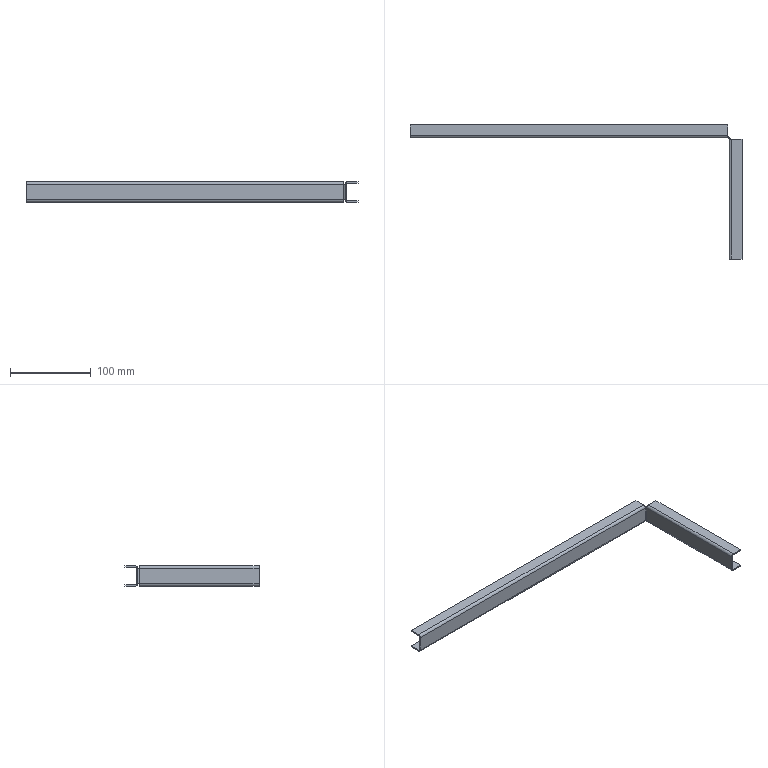Part | NX | features solid 2 | 1 solid | 34 faces | box 411 x 166 x 25 mm | volume 42432 mm3 | plane 24 | cylinder 10 | commonest cylinder face diameters 3 x5 6 x5
STEP:
#1=CARTESIAN_POINT('',(1091.,510.5,389.));
#2=VERTEX_POINT('',#1);
#3=CARTESIAN_POINT('',(1091.,509.,390.5));
#4=VERTEX_POINT('',#3);
#5=CARTESIAN_POINT('',(1091.,510.5,390.5));
#6=DIRECTION('',(-1.,0.,0.));
#7=DIRECTION('',(0.,0.,1.));
#8=AXIS2_PLACEMENT_3D('',#5,#6,#7);
#9=CIRCLE('',#8,1.5);
#10=EDGE_CURVE('',#2,#4,#9,.T.);
#11=ORIENTED_EDGE('',*,*,#10,.F.);
#12=CARTESIAN_POINT('',(697.5,510.5,389.));
#13=VERTEX_POINT('',#12);
#14=CARTESIAN_POINT('',(1091.,510.5,389.));
#15=DIRECTION('',(-1.,0.,0.));
#16=VECTOR('',#15,1000.);
#17=LINE('',#14,#16);
#18=EDGE_CURVE('',#2,#13,#17,.T.);
#19=ORIENTED_EDGE('',*,*,#18,.T.);
#20=CARTESIAN_POINT('',(697.5,509.,390.5));
#21=VERTEX_POINT('',#20);
#22=CARTESIAN_POINT('',(697.5,510.5,390.5));
#23=DIRECTION('',(1.,0.,0.));
#24=DIRECTION('',(0.,0.,1.));
#25=AXIS2_PLACEMENT_3D('',#22,#23,#24);
#26=CIRCLE('',#25,1.5);
#27=EDGE_CURVE('',#21,#13,#26,.T.);
#28=ORIENTED_EDGE('',*,*,#27,.F.);
#29=CARTESIAN_POINT('',(697.5,509.,390.5));
#30=DIRECTION('',(1.,0.,0.));
#31=VECTOR('',#30,1000.);
#32=LINE('',#29,#31);
#33=EDGE_CURVE('',#21,#4,#32,.T.);
#34=ORIENTED_EDGE('',*,*,#33,.T.);
#35=EDGE_LOOP('',(#11,#19,#28,#34));
#36=FACE_BOUND('',#35,.T.);
#37=CARTESIAN_POINT('',(697.5,510.5,390.5));
#38=DIRECTION('',(-1.,0.,0.));
#39=DIRECTION('',(0.,1.,0.));
#40=AXIS2_PLACEMENT_3D('',#37,#38,#39);
#41=CYLINDRICAL_SURFACE('',#40,1.5);
#42=ADVANCED_FACE('',(#36),#41,.F.);
#43=CARTESIAN_POINT('',(1091.,510.5,387.5));
#44=VERTEX_POINT('',#43);
#45=CARTESIAN_POINT('',(1091.,507.5,390.5));
#46=VERTEX_POINT('',#45);
#47=CARTESIAN_POINT('',(1091.,510.5,390.5));
#48=DIRECTION('',(-1.,0.,0.));
#49=DIRECTION('',(0.,1.,0.));
#50=AXIS2_PLACEMENT_3D('',#47,#48,#49);
#51=CIRCLE('',#50,3.);
#52=EDGE_CURVE('',#44,#46,#51,.T.);
#53=ORIENTED_EDGE('',*,*,#52,.T.);
#54=CARTESIAN_POINT('',(697.5,507.5,390.5));
#55=VERTEX_POINT('',#54);
#56=CARTESIAN_POINT('',(1091.,507.5,390.5));
#57=DIRECTION('',(1.,0.,0.));
#58=VECTOR('',#57,1000.);
#59=LINE('',#56,#58);
#60=EDGE_CURVE('',#55,#46,#59,.T.);
#61=ORIENTED_EDGE('',*,*,#60,.F.);
#62=CARTESIAN_POINT('',(697.5,510.5,387.5));
#63=VERTEX_POINT('',#62);
#64=CARTESIAN_POINT('',(697.5,510.5,390.5));
#65=DIRECTION('',(1.,0.,0.));
#66=DIRECTION('',(0.,1.,0.));
#67=AXIS2_PLACEMENT_3D('',#64,#65,#66);
#68=CIRCLE('',#67,3.);
#69=EDGE_CURVE('',#55,#63,#68,.T.);
#70=ORIENTED_EDGE('',*,*,#69,.T.);
#71=CARTESIAN_POINT('',(1091.,510.5,387.5));
#72=DIRECTION('',(-1.,0.,0.));
#73=VECTOR('',#72,1000.);
#74=LINE('',#71,#73);
#75=EDGE_CURVE('',#44,#63,#74,.T.);
#76=ORIENTED_EDGE('',*,*,#75,.F.);
#77=EDGE_LOOP('',(#53,#61,#70,#76));
#78=FACE_BOUND('',#77,.T.);
#79=CARTESIAN_POINT('',(697.5,510.5,390.5));
#80=DIRECTION('',(-1.,0.,0.));
#81=DIRECTION('',(0.,1.,0.));
#82=AXIS2_PLACEMENT_3D('',#79,#80,#81);
#83=CYLINDRICAL_SURFACE('',#82,3.);
#84=ADVANCED_FACE('',(#78),#83,.T.);
#85=CARTESIAN_POINT('',(697.5,523.5,389.));
#86=VERTEX_POINT('',#85);
#87=CARTESIAN_POINT('',(697.5,523.5,389.));
#88=DIRECTION('',(0.,-1.,0.));
#89=VECTOR('',#88,1000.);
#90=LINE('',#87,#89);
#91=EDGE_CURVE('',#86,#13,#90,.T.);
#92=ORIENTED_EDGE('',*,*,#91,.T.);
#93=ORIENTED_EDGE('',*,*,#18,.F.);
#94=CARTESIAN_POINT('',(1091.,523.5,389.));
#95=VERTEX_POINT('',#94);
#96=CARTESIAN_POINT('',(1091.,523.5,389.));
#97=DIRECTION('',(0.,-1.,0.));
#98=VECTOR('',#97,1000.);
#99=LINE('',#96,#98);
#100=EDGE_CURVE('',#95,#2,#99,.T.);
#101=ORIENTED_EDGE('',*,*,#100,.F.);
#102=CARTESIAN_POINT('',(1091.,523.5,389.));
#103=DIRECTION('',(-1.,0.,0.));
#104=VECTOR('',#103,1000.);
#105=LINE('',#102,#104);
#106=EDGE_CURVE('',#95,#86,#105,.T.);
#107=ORIENTED_EDGE('',*,*,#106,.T.);
#108=EDGE_LOOP('',(#92,#93,#101,#107));
#109=FACE_BOUND('',#108,.T.);
#110=CARTESIAN_POINT('',(1091.,523.5,389.));
#111=DIRECTION('',(0.,0.,-1.));
#112=DIRECTION('',(-1.,0.,0.));
#113=AXIS2_PLACEMENT_3D('',#110,#111,#112);
#114=PLANE('',#113);
#115=ADVANCED_FACE('',(#109),#114,.F.);
#116=CARTESIAN_POINT('',(697.5,523.5,387.5));
#117=VERTEX_POINT('',#116);
#118=CARTESIAN_POINT('',(697.5,523.5,387.5));
#119=DIRECTION('',(0.,-1.,0.));
#120=VECTOR('',#119,1000.);
#121=LINE('',#118,#120);
#122=EDGE_CURVE('',#117,#63,#121,.T.);
#123=ORIENTED_EDGE('',*,*,#122,.F.);
#124=CARTESIAN_POINT('',(1091.,523.5,387.5));
#125=VERTEX_POINT('',#124);
#126=CARTESIAN_POINT('',(1091.,523.5,387.5));
#127=DIRECTION('',(-1.,0.,0.));
#128=VECTOR('',#127,1000.);
#129=LINE('',#126,#128);
#130=EDGE_CURVE('',#125,#117,#129,.T.);
#131=ORIENTED_EDGE('',*,*,#130,.F.);
#132=CARTESIAN_POINT('',(1091.,523.5,387.5));
#133=DIRECTION('',(0.,-1.,0.));
#134=VECTOR('',#133,1000.);
#135=LINE('',#132,#134);
#136=EDGE_CURVE('',#125,#44,#135,.T.);
#137=ORIENTED_EDGE('',*,*,#136,.T.);
#138=ORIENTED_EDGE('',*,*,#75,.T.);
#139=EDGE_LOOP('',(#123,#131,#137,#138));
#140=FACE_BOUND('',#139,.T.);
#141=CARTESIAN_POINT('',(1091.,523.5,387.5));
#142=DIRECTION('',(0.,0.,-1.));
#143=DIRECTION('',(-1.,0.,0.));
#144=AXIS2_PLACEMENT_3D('',#141,#142,#143);
#145=PLANE('',#144);
#146=ADVANCED_FACE('',(#140),#145,.T.);
#147=ORIENTED_EDGE('',*,*,#106,.F.);
#148=CARTESIAN_POINT('',(1091.,523.5,387.5));
#149=DIRECTION('',(0.,0.,-1.));
#150=VECTOR('',#149,1000.);
#151=LINE('',#148,#150);
#152=EDGE_CURVE('',#95,#125,#151,.T.);
#153=ORIENTED_EDGE('',*,*,#152,.T.);
#154=ORIENTED_EDGE('',*,*,#130,.T.);
#155=CARTESIAN_POINT('',(697.5,523.5,387.5));
#156=DIRECTION('',(0.,0.,-1.));
#157=VECTOR('',#156,1000.);
#158=LINE('',#155,#157);
#159=EDGE_CURVE('',#86,#117,#158,.T.);
#160=ORIENTED_EDGE('',*,*,#159,.F.);
#161=EDGE_LOOP('',(#147,#153,#154,#160));
#162=FACE_BOUND('',#161,.T.);
#163=CARTESIAN_POINT('',(1091.,523.5,387.5));
#164=DIRECTION('',(0.,-1.,0.));
#165=DIRECTION('',(-1.,0.,0.));
#166=AXIS2_PLACEMENT_3D('',#163,#164,#165);
#167=PLANE('',#166);
#168=ADVANCED_FACE('',(#162),#167,.F.);
#169=ORIENTED_EDGE('',*,*,#152,.F.);
#170=ORIENTED_EDGE('',*,*,#100,.T.);
#171=ORIENTED_EDGE('',*,*,#10,.T.);
#172=CARTESIAN_POINT('',(1091.,507.5,390.5));
#173=DIRECTION('',(0.,-1.,0.));
#174=VECTOR('',#173,1000.);
#175=LINE('',#172,#174);
#176=EDGE_CURVE('',#4,#46,#175,.T.);
#177=ORIENTED_EDGE('',*,*,#176,.T.);
#178=ORIENTED_EDGE('',*,*,#52,.F.);
#179=ORIENTED_EDGE('',*,*,#136,.F.);
#180=EDGE_LOOP('',(#169,#170,#171,#177,#178,#179));
#181=FACE_BOUND('',#180,.T.);
#182=CARTESIAN_POINT('',(1091.,523.5,387.5));
#183=DIRECTION('',(1.,0.,0.));
#184=DIRECTION('',(0.,0.,-1.));
#185=AXIS2_PLACEMENT_3D('',#182,#183,#184);
#186=PLANE('',#185);
#187=ADVANCED_FACE('',(#181),#186,.T.);
#188=CARTESIAN_POINT('',(1095.5,357.5,389.));
#189=VERTEX_POINT('',#188);
#190=CARTESIAN_POINT('',(1094.,357.5,390.5));
#191=VERTEX_POINT('',#190);
#192=CARTESIAN_POINT('',(1095.5,357.5,390.5));
#193=DIRECTION('',(0.,1.,0.));
#194=DIRECTION('',(0.,0.,-1.));
#195=AXIS2_PLACEMENT_3D('',#192,#193,#194);
#196=CIRCLE('',#195,1.5);
#197=EDGE_CURVE('',#189,#191,#196,.T.);
#198=ORIENTED_EDGE('',*,*,#197,.F.);
#199=CARTESIAN_POINT('',(1095.5,506.,389.));
#200=VERTEX_POINT('',#199);
#201=CARTESIAN_POINT('',(1095.5,357.5,389.));
#202=DIRECTION('',(0.,1.,0.));
#203=VECTOR('',#202,1000.);
#204=LINE('',#201,#203);
#205=EDGE_CURVE('',#189,#200,#204,.T.);
#206=ORIENTED_EDGE('',*,*,#205,.T.);
#207=CARTESIAN_POINT('',(1094.,506.,390.5));
#208=VERTEX_POINT('',#207);
#209=CARTESIAN_POINT('',(1095.5,506.,390.5));
#210=DIRECTION('',(0.,-1.,0.));
#211=DIRECTION('',(0.,0.,-1.));
#212=AXIS2_PLACEMENT_3D('',#209,#210,#211);
#213=CIRCLE('',#212,1.5);
#214=EDGE_CURVE('',#208,#200,#213,.T.);
#215=ORIENTED_EDGE('',*,*,#214,.F.);
#216=CARTESIAN_POINT('',(1094.,506.,390.5));
#217=DIRECTION('',(0.,-1.,0.));
#218=VECTOR('',#217,1000.);
#219=LINE('',#216,#218);
#220=EDGE_CURVE('',#208,#191,#219,.T.);
#221=ORIENTED_EDGE('',*,*,#220,.T.);
#222=EDGE_LOOP('',(#198,#206,#215,#221));
#223=FACE_BOUND('',#222,.T.);
#224=CARTESIAN_POINT('',(1095.5,506.,390.5));
#225=DIRECTION('',(0.,1.,0.));
#226=DIRECTION('',(1.,0.,0.));
#227=AXIS2_PLACEMENT_3D('',#224,#225,#226);
#228=CYLINDRICAL_SURFACE('',#227,1.5);
#229=ADVANCED_FACE('',(#223),#228,.F.);
#230=CARTESIAN_POINT('',(1095.5,357.5,387.5));
#231=VERTEX_POINT('',#230);
#232=CARTESIAN_POINT('',(1092.5,357.5,390.5));
#233=VERTEX_POINT('',#232);
#234=CARTESIAN_POINT('',(1095.5,357.5,390.5));
#235=DIRECTION('',(0.,1.,0.));
#236=DIRECTION('',(1.,0.,0.));
#237=AXIS2_PLACEMENT_3D('',#234,#235,#236);
#238=CIRCLE('',#237,3.);
#239=EDGE_CURVE('',#231,#233,#238,.T.);
#240=ORIENTED_EDGE('',*,*,#239,.T.);
#241=CARTESIAN_POINT('',(1092.5,506.,390.5));
#242=VERTEX_POINT('',#241);
#243=CARTESIAN_POINT('',(1092.5,357.5,390.5));
#244=DIRECTION('',(0.,-1.,0.));
#245=VECTOR('',#244,1000.);
#246=LINE('',#243,#245);
#247=EDGE_CURVE('',#242,#233,#246,.T.);
#248=ORIENTED_EDGE('',*,*,#247,.F.);
#249=CARTESIAN_POINT('',(1095.5,506.,387.5));
#250=VERTEX_POINT('',#249);
#251=CARTESIAN_POINT('',(1095.5,506.,390.5));
#252=DIRECTION('',(0.,-1.,0.));
#253=DIRECTION('',(1.,0.,0.));
#254=AXIS2_PLACEMENT_3D('',#251,#252,#253);
#255=CIRCLE('',#254,3.);
#256=EDGE_CURVE('',#242,#250,#255,.T.);
#257=ORIENTED_EDGE('',*,*,#256,.T.);
#258=CARTESIAN_POINT('',(1095.5,357.5,387.5));
#259=DIRECTION('',(0.,1.,0.));
#260=VECTOR('',#259,1000.);
#261=LINE('',#258,#260);
#262=EDGE_CURVE('',#231,#250,#261,.T.);
#263=ORIENTED_EDGE('',*,*,#262,.F.);
#264=EDGE_LOOP('',(#240,#248,#257,#263));
#265=FACE_BOUND('',#264,.T.);
#266=CARTESIAN_POINT('',(1095.5,506.,390.5));
#267=DIRECTION('',(0.,1.,0.));
#268=DIRECTION('',(1.,0.,0.));
#269=AXIS2_PLACEMENT_3D('',#266,#267,#268);
#270=CYLINDRICAL_SURFACE('',#269,3.);
#271=ADVANCED_FACE('',(#265),#270,.T.);
#272=CARTESIAN_POINT('',(1108.5,506.,389.));
#273=VERTEX_POINT('',#272);
#274=CARTESIAN_POINT('',(1108.5,506.,389.));
#275=DIRECTION('',(-1.,0.,0.));
#276=VECTOR('',#275,1000.);
#277=LINE('',#274,#276);
#278=EDGE_CURVE('',#273,#200,#277,.T.);
#279=ORIENTED_EDGE('',*,*,#278,.T.);
#280=ORIENTED_EDGE('',*,*,#205,.F.);
#281=CARTESIAN_POINT('',(1108.5,357.5,389.));
#282=VERTEX_POINT('',#281);
#283=CARTESIAN_POINT('',(1108.5,357.5,389.));
#284=DIRECTION('',(-1.,0.,0.));
#285=VECTOR('',#284,1000.);
#286=LINE('',#283,#285);
#287=EDGE_CURVE('',#282,#189,#286,.T.);
#288=ORIENTED_EDGE('',*,*,#287,.F.);
#289=CARTESIAN_POINT('',(1108.5,357.5,389.));
#290=DIRECTION('',(0.,1.,0.));
#291=VECTOR('',#290,1000.);
#292=LINE('',#289,#291);
#293=EDGE_CURVE('',#282,#273,#292,.T.);
#294=ORIENTED_EDGE('',*,*,#293,.T.);
#295=EDGE_LOOP('',(#279,#280,#288,#294));
#296=FACE_BOUND('',#295,.T.);
#297=CARTESIAN_POINT('',(1108.5,357.5,389.));
#298=DIRECTION('',(0.,0.,-1.));
#299=DIRECTION('',(-1.,0.,0.));
#300=AXIS2_PLACEMENT_3D('',#297,#298,#299);
#301=PLANE('',#300);
#302=ADVANCED_FACE('',(#296),#301,.F.);
#303=CARTESIAN_POINT('',(1108.5,506.,387.5));
#304=VERTEX_POINT('',#303);
#305=CARTESIAN_POINT('',(1108.5,506.,387.5));
#306=DIRECTION('',(-1.,0.,0.));
#307=VECTOR('',#306,1000.);
#308=LINE('',#305,#307);
#309=EDGE_CURVE('',#304,#250,#308,.T.);
#310=ORIENTED_EDGE('',*,*,#309,.F.);
#311=CARTESIAN_POINT('',(1108.5,357.5,387.5));
#312=VERTEX_POINT('',#311);
#313=CARTESIAN_POINT('',(1108.5,357.5,387.5));
#314=DIRECTION('',(0.,1.,0.));
#315=VECTOR('',#314,1000.);
#316=LINE('',#313,#315);
#317=EDGE_CURVE('',#312,#304,#316,.T.);
#318=ORIENTED_EDGE('',*,*,#317,.F.);
#319=CARTESIAN_POINT('',(1108.5,357.5,387.5));
#320=DIRECTION('',(-1.,0.,0.));
#321=VECTOR('',#320,1000.);
#322=LINE('',#319,#321);
#323=EDGE_CURVE('',#312,#231,#322,.T.);
#324=ORIENTED_EDGE('',*,*,#323,.T.);
#325=ORIENTED_EDGE('',*,*,#262,.T.);
#326=EDGE_LOOP('',(#310,#318,#324,#325));
#327=FACE_BOUND('',#326,.T.);
#328=CARTESIAN_POINT('',(1108.5,357.5,387.5));
#329=DIRECTION('',(0.,0.,-1.));
#330=DIRECTION('',(-1.,0.,0.));
#331=AXIS2_PLACEMENT_3D('',#328,#329,#330);
#332=PLANE('',#331);
#333=ADVANCED_FACE('',(#327),#332,.T.);
#334=ORIENTED_EDGE('',*,*,#293,.F.);
#335=CARTESIAN_POINT('',(1108.5,357.5,387.5));
#336=DIRECTION('',(0.,0.,-1.));
#337=VECTOR('',#336,1000.);
#338=LINE('',#335,#337);
#339=EDGE_CURVE('',#282,#312,#338,.T.);
#340=ORIENTED_EDGE('',*,*,#339,.T.);
#341=ORIENTED_EDGE('',*,*,#317,.T.);
#342=CARTESIAN_POINT('',(1108.5,506.,387.5));
#343=DIRECTION('',(0.,0.,-1.));
#344=VECTOR('',#343,1000.);
#345=LINE('',#342,#344);
#346=EDGE_CURVE('',#273,#304,#345,.T.);
#347=ORIENTED_EDGE('',*,*,#346,.F.);
#348=EDGE_LOOP('',(#334,#340,#341,#347));
#349=FACE_BOUND('',#348,.T.);
#350=CARTESIAN_POINT('',(1108.5,357.5,387.5));
#351=DIRECTION('',(-1.,0.,0.));
#352=DIRECTION('',(0.,0.,1.));
#353=AXIS2_PLACEMENT_3D('',#350,#351,#352);
#354=PLANE('',#353);
#355=ADVANCED_FACE('',(#349),#354,.F.);
#356=ORIENTED_EDGE('',*,*,#309,.T.);
#357=ORIENTED_EDGE('',*,*,#256,.F.);
#358=CARTESIAN_POINT('',(1092.5,506.,390.5));
#359=DIRECTION('',(-1.,0.,0.));
#360=VECTOR('',#359,1000.);
#361=LINE('',#358,#360);
#362=EDGE_CURVE('',#208,#242,#361,.T.);
#363=ORIENTED_EDGE('',*,*,#362,.F.);
#364=ORIENTED_EDGE('',*,*,#214,.T.);
#365=ORIENTED_EDGE('',*,*,#278,.F.);
#366=ORIENTED_EDGE('',*,*,#346,.T.);
#367=EDGE_LOOP('',(#356,#357,#363,#364,#365,#366));
#368=FACE_BOUND('',#367,.T.);
#369=CARTESIAN_POINT('',(1108.5,506.,387.5));
#370=DIRECTION('',(0.,-1.,0.));
#371=DIRECTION('',(-1.,0.,0.));
#372=AXIS2_PLACEMENT_3D('',#369,#370,#371);
#373=PLANE('',#372);
#374=ADVANCED_FACE('',(#368),#373,.F.);
#375=CARTESIAN_POINT('',(1091.,506.,390.5));
#376=DIRECTION('',(0.,0.,-1.));
#377=DIRECTION('',(0.,1.,0.));
#378=AXIS2_PLACEMENT_3D('',#375,#376,#377);
#379=CIRCLE('',#378,1.5);
#380=EDGE_CURVE('',#46,#242,#379,.T.);
#381=ORIENTED_EDGE('',*,*,#380,.F.);
#382=ORIENTED_EDGE('',*,*,#176,.F.);
#383=CARTESIAN_POINT('',(1091.,506.,390.5));
#384=DIRECTION('',(0.,0.,-1.));
#385=DIRECTION('',(0.,1.,0.));
#386=AXIS2_PLACEMENT_3D('',#383,#384,#385);
#387=CIRCLE('',#386,3.);
#388=EDGE_CURVE('',#4,#208,#387,.T.);
#389=ORIENTED_EDGE('',*,*,#388,.T.);
#390=ORIENTED_EDGE('',*,*,#362,.T.);
#391=EDGE_LOOP('',(#381,#382,#389,#390));
#392=FACE_BOUND('',#391,.T.);
#393=CARTESIAN_POINT('',(1092.5,357.5,390.5));
#394=DIRECTION('',(0.,0.,1.));
#395=DIRECTION('',(0.,-1.,0.));
#396=AXIS2_PLACEMENT_3D('',#393,#394,#395);
#397=PLANE('',#396);
#398=ADVANCED_FACE('',(#392),#397,.F.);
#399=CARTESIAN_POINT('',(697.5,510.5,411.));
#400=VERTEX_POINT('',#399);
#401=CARTESIAN_POINT('',(697.5,509.,409.5));
#402=VERTEX_POINT('',#401);
#403=CARTESIAN_POINT('',(697.5,510.5,409.5));
#404=DIRECTION('',(1.,0.,0.));
#405=DIRECTION('',(0.,1.,0.));
#406=AXIS2_PLACEMENT_3D('',#403,#404,#405);
#407=CIRCLE('',#406,1.5);
#408=EDGE_CURVE('',#400,#402,#407,.T.);
#409=ORIENTED_EDGE('',*,*,#408,.F.);
#410=CARTESIAN_POINT('',(1091.,510.5,411.));
#411=VERTEX_POINT('',#410);
#412=CARTESIAN_POINT('',(1091.,510.5,411.));
#413=DIRECTION('',(-1.,0.,0.));
#414=VECTOR('',#413,1000.);
#415=LINE('',#412,#414);
#416=EDGE_CURVE('',#411,#400,#415,.T.);
#417=ORIENTED_EDGE('',*,*,#416,.F.);
#418=CARTESIAN_POINT('',(1091.,509.,409.5));
#419=VERTEX_POINT('',#418);
#420=CARTESIAN_POINT('',(1091.,510.5,409.5));
#421=DIRECTION('',(-1.,0.,0.));
#422=DIRECTION('',(0.,1.,0.));
#423=AXIS2_PLACEMENT_3D('',#420,#421,#422);
#424=CIRCLE('',#423,1.5);
#425=EDGE_CURVE('',#419,#411,#424,.T.);
#426=ORIENTED_EDGE('',*,*,#425,.F.);
#427=CARTESIAN_POINT('',(1091.,509.,409.5));
#428=DIRECTION('',(-1.,0.,0.));
#429=VECTOR('',#428,1000.);
#430=LINE('',#427,#429);
#431=EDGE_CURVE('',#419,#402,#430,.T.);
#432=ORIENTED_EDGE('',*,*,#431,.T.);
#433=EDGE_LOOP('',(#409,#417,#426,#432));
#434=FACE_BOUND('',#433,.T.);
#435=CARTESIAN_POINT('',(1091.,510.5,409.5));
#436=DIRECTION('',(1.,0.,0.));
#437=DIRECTION('',(0.,1.,0.));
#438=AXIS2_PLACEMENT_3D('',#435,#436,#437);
#439=CYLINDRICAL_SURFACE('',#438,1.5);
#440=ADVANCED_FACE('',(#434),#439,.F.);
#441=CARTESIAN_POINT('',(697.5,510.5,412.5));
#442=VERTEX_POINT('',#441);
#443=CARTESIAN_POINT('',(697.5,507.5,409.5));
#444=VERTEX_POINT('',#443);
#445=CARTESIAN_POINT('',(697.5,510.5,409.5));
#446=DIRECTION('',(1.,0.,0.));
#447=DIRECTION('',(0.,1.,0.));
#448=AXIS2_PLACEMENT_3D('',#445,#446,#447);
#449=CIRCLE('',#448,3.);
#450=EDGE_CURVE('',#442,#444,#449,.T.);
#451=ORIENTED_EDGE('',*,*,#450,.T.);
#452=CARTESIAN_POINT('',(1091.,507.5,409.5));
#453=VERTEX_POINT('',#452);
#454=CARTESIAN_POINT('',(697.5,507.5,409.5));
#455=DIRECTION('',(-1.,0.,0.));
#456=VECTOR('',#455,1000.);
#457=LINE('',#454,#456);
#458=EDGE_CURVE('',#453,#444,#457,.T.);
#459=ORIENTED_EDGE('',*,*,#458,.F.);
#460=CARTESIAN_POINT('',(1091.,510.5,412.5));
#461=VERTEX_POINT('',#460);
#462=CARTESIAN_POINT('',(1091.,510.5,409.5));
#463=DIRECTION('',(-1.,0.,0.));
#464=DIRECTION('',(0.,1.,0.));
#465=AXIS2_PLACEMENT_3D('',#462,#463,#464);
#466=CIRCLE('',#465,3.);
#467=EDGE_CURVE('',#453,#461,#466,.T.);
#468=ORIENTED_EDGE('',*,*,#467,.T.);
#469=CARTESIAN_POINT('',(1091.,510.5,412.5));
#470=DIRECTION('',(-1.,0.,0.));
#471=VECTOR('',#470,1000.);
#472=LINE('',#469,#471);
#473=EDGE_CURVE('',#461,#442,#472,.T.);
#474=ORIENTED_EDGE('',*,*,#473,.T.);
#475=EDGE_LOOP('',(#451,#459,#468,#474));
#476=FACE_BOUND('',#475,.T.);
#477=CARTESIAN_POINT('',(1091.,510.5,409.5));
#478=DIRECTION('',(1.,0.,0.));
#479=DIRECTION('',(0.,1.,0.));
#480=AXIS2_PLACEMENT_3D('',#477,#478,#479);
#481=CYLINDRICAL_SURFACE('',#480,3.);
#482=ADVANCED_FACE('',(#476),#481,.T.);
#483=CARTESIAN_POINT('',(697.5,523.5,411.));
#484=VERTEX_POINT('',#483);
#485=CARTESIAN_POINT('',(697.5,507.5,411.));
#486=DIRECTION('',(0.,1.,0.));
#487=VECTOR('',#486,1000.);
#488=LINE('',#485,#487);
#489=EDGE_CURVE('',#400,#484,#488,.T.);
#490=ORIENTED_EDGE('',*,*,#489,.T.);
#491=CARTESIAN_POINT('',(1091.,523.5,411.));
#492=VERTEX_POINT('',#491);
#493=CARTESIAN_POINT('',(1091.,523.5,411.));
#494=DIRECTION('',(-1.,0.,0.));
#495=VECTOR('',#494,1000.);
#496=LINE('',#493,#495);
#497=EDGE_CURVE('',#492,#484,#496,.T.);
#498=ORIENTED_EDGE('',*,*,#497,.F.);
#499=CARTESIAN_POINT('',(1091.,507.5,411.));
#500=DIRECTION('',(0.,1.,0.));
#501=VECTOR('',#500,1000.);
#502=LINE('',#499,#501);
#503=EDGE_CURVE('',#411,#492,#502,.T.);
#504=ORIENTED_EDGE('',*,*,#503,.F.);
#505=ORIENTED_EDGE('',*,*,#416,.T.);
#506=EDGE_LOOP('',(#490,#498,#504,#505));
#507=FACE_BOUND('',#506,.T.);
#508=CARTESIAN_POINT('',(1091.,507.5,411.));
#509=DIRECTION('',(0.,0.,1.));
#510=DIRECTION('',(0.,-1.,0.));
#511=AXIS2_PLACEMENT_3D('',#508,#509,#510);
#512=PLANE('',#511);
#513=ADVANCED_FACE('',(#507),#512,.F.);
#514=CARTESIAN_POINT('',(697.5,523.5,412.5));
#515=VERTEX_POINT('',#514);
#516=CARTESIAN_POINT('',(697.5,507.5,412.5));
#517=DIRECTION('',(0.,1.,0.));
#518=VECTOR('',#517,1000.);
#519=LINE('',#516,#518);
#520=EDGE_CURVE('',#442,#515,#519,.T.);
#521=ORIENTED_EDGE('',*,*,#520,.F.);
#522=ORIENTED_EDGE('',*,*,#473,.F.);
#523=CARTESIAN_POINT('',(1091.,523.5,412.5));
#524=VERTEX_POINT('',#523);
#525=CARTESIAN_POINT('',(1091.,507.5,412.5));
#526=DIRECTION('',(0.,1.,0.));
#527=VECTOR('',#526,1000.);
#528=LINE('',#525,#527);
#529=EDGE_CURVE('',#461,#524,#528,.T.);
#530=ORIENTED_EDGE('',*,*,#529,.T.);
#531=CARTESIAN_POINT('',(1091.,523.5,412.5));
#532=DIRECTION('',(-1.,0.,0.));
#533=VECTOR('',#532,1000.);
#534=LINE('',#531,#533);
#535=EDGE_CURVE('',#524,#515,#534,.T.);
#536=ORIENTED_EDGE('',*,*,#535,.T.);
#537=EDGE_LOOP('',(#521,#522,#530,#536));
#538=FACE_BOUND('',#537,.T.);
#539=CARTESIAN_POINT('',(1091.,507.5,412.5));
#540=DIRECTION('',(0.,0.,1.));
#541=DIRECTION('',(0.,-1.,0.));
#542=AXIS2_PLACEMENT_3D('',#539,#540,#541);
#543=PLANE('',#542);
#544=ADVANCED_FACE('',(#538),#543,.T.);
#545=CARTESIAN_POINT('',(1091.,523.5,412.5));
#546=DIRECTION('',(0.,0.,1.));
#547=VECTOR('',#546,1000.);
#548=LINE('',#545,#547);
#549=EDGE_CURVE('',#492,#524,#548,.T.);
#550=ORIENTED_EDGE('',*,*,#549,.F.);
#551=ORIENTED_EDGE('',*,*,#497,.T.);
#552=CARTESIAN_POINT('',(697.5,523.5,412.5));
#553=DIRECTION('',(0.,0.,1.));
#554=VECTOR('',#553,1000.);
#555=LINE('',#552,#554);
#556=EDGE_CURVE('',#484,#515,#555,.T.);
#557=ORIENTED_EDGE('',*,*,#556,.T.);
#558=ORIENTED_EDGE('',*,*,#535,.F.);
#559=EDGE_LOOP('',(#550,#551,#557,#558));
#560=FACE_BOUND('',#559,.T.);
#561=CARTESIAN_POINT('',(1091.,523.5,412.5));
#562=DIRECTION('',(0.,1.,0.));
#563=DIRECTION('',(1.,0.,0.));
#564=AXIS2_PLACEMENT_3D('',#561,#562,#563);
#565=PLANE('',#564);
#566=ADVANCED_FACE('',(#560),#565,.T.);
#567=ORIENTED_EDGE('',*,*,#529,.F.);
#568=ORIENTED_EDGE('',*,*,#467,.F.);
#569=CARTESIAN_POINT('',(1091.,507.5,409.5));
#570=DIRECTION('',(0.,-1.,0.));
#571=VECTOR('',#570,1000.);
#572=LINE('',#569,#571);
#573=EDGE_CURVE('',#419,#453,#572,.T.);
#574=ORIENTED_EDGE('',*,*,#573,.F.);
#575=ORIENTED_EDGE('',*,*,#425,.T.);
#576=ORIENTED_EDGE('',*,*,#503,.T.);
#577=ORIENTED_EDGE('',*,*,#549,.T.);
#578=EDGE_LOOP('',(#567,#568,#574,#575,#576,#577));
#579=FACE_BOUND('',#578,.T.);
#580=CARTESIAN_POINT('',(1091.,507.5,412.5));
#581=DIRECTION('',(1.,0.,0.));
#582=DIRECTION('',(0.,0.,-1.));
#583=AXIS2_PLACEMENT_3D('',#580,#581,#582);
#584=PLANE('',#583);
#585=ADVANCED_FACE('',(#579),#584,.T.);
#586=CARTESIAN_POINT('',(1095.5,506.,411.));
#587=VERTEX_POINT('',#586);
#588=CARTESIAN_POINT('',(1094.,506.,409.5));
#589=VERTEX_POINT('',#588);
#590=CARTESIAN_POINT('',(1095.5,506.,409.5));
#591=DIRECTION('',(0.,-1.,0.));
#592=DIRECTION('',(0.,0.,1.));
#593=AXIS2_PLACEMENT_3D('',#590,#591,#592);
#594=CIRCLE('',#593,1.5);
#595=EDGE_CURVE('',#587,#589,#594,.T.);
#596=ORIENTED_EDGE('',*,*,#595,.F.);
#597=CARTESIAN_POINT('',(1095.5,357.5,411.));
#598=VERTEX_POINT('',#597);
#599=CARTESIAN_POINT('',(1095.5,357.5,411.));
#600=DIRECTION('',(0.,1.,0.));
#601=VECTOR('',#600,1000.);
#602=LINE('',#599,#601);
#603=EDGE_CURVE('',#598,#587,#602,.T.);
#604=ORIENTED_EDGE('',*,*,#603,.F.);
#605=CARTESIAN_POINT('',(1094.,357.5,409.5));
#606=VERTEX_POINT('',#605);
#607=CARTESIAN_POINT('',(1095.5,357.5,409.5));
#608=DIRECTION('',(0.,1.,0.));
#609=DIRECTION('',(0.,0.,1.));
#610=AXIS2_PLACEMENT_3D('',#607,#608,#609);
#611=CIRCLE('',#610,1.5);
#612=EDGE_CURVE('',#606,#598,#611,.T.);
#613=ORIENTED_EDGE('',*,*,#612,.F.);
#614=CARTESIAN_POINT('',(1094.,357.5,409.5));
#615=DIRECTION('',(0.,1.,0.));
#616=VECTOR('',#615,1000.);
#617=LINE('',#614,#616);
#618=EDGE_CURVE('',#606,#589,#617,.T.);
#619=ORIENTED_EDGE('',*,*,#618,.T.);
#620=EDGE_LOOP('',(#596,#604,#613,#619));
#621=FACE_BOUND('',#620,.T.);
#622=CARTESIAN_POINT('',(1095.5,357.5,409.5));
#623=DIRECTION('',(0.,-1.,0.));
#624=DIRECTION('',(1.,0.,0.));
#625=AXIS2_PLACEMENT_3D('',#622,#623,#624);
#626=CYLINDRICAL_SURFACE('',#625,1.5);
#627=ADVANCED_FACE('',(#621),#626,.F.);
#628=CARTESIAN_POINT('',(1095.5,506.,412.5));
#629=VERTEX_POINT('',#628);
#630=CARTESIAN_POINT('',(1092.5,506.,409.5));
#631=VERTEX_POINT('',#630);
#632=CARTESIAN_POINT('',(1095.5,506.,409.5));
#633=DIRECTION('',(0.,-1.,0.));
#634=DIRECTION('',(1.,0.,0.));
#635=AXIS2_PLACEMENT_3D('',#632,#633,#634);
#636=CIRCLE('',#635,3.);
#637=EDGE_CURVE('',#629,#631,#636,.T.);
#638=ORIENTED_EDGE('',*,*,#637,.T.);
#639=CARTESIAN_POINT('',(1092.5,357.5,409.5));
#640=VERTEX_POINT('',#639);
#641=CARTESIAN_POINT('',(1092.5,506.,409.5));
#642=DIRECTION('',(0.,1.,0.));
#643=VECTOR('',#642,1000.);
#644=LINE('',#641,#643);
#645=EDGE_CURVE('',#640,#631,#644,.T.);
#646=ORIENTED_EDGE('',*,*,#645,.F.);
#647=CARTESIAN_POINT('',(1095.5,357.5,412.5));
#648=VERTEX_POINT('',#647);
#649=CARTESIAN_POINT('',(1095.5,357.5,409.5));
#650=DIRECTION('',(0.,1.,0.));
#651=DIRECTION('',(1.,0.,0.));
#652=AXIS2_PLACEMENT_3D('',#649,#650,#651);
#653=CIRCLE('',#652,3.);
#654=EDGE_CURVE('',#640,#648,#653,.T.);
#655=ORIENTED_EDGE('',*,*,#654,.T.);
#656=CARTESIAN_POINT('',(1095.5,357.5,412.5));
#657=DIRECTION('',(0.,1.,0.));
#658=VECTOR('',#657,1000.);
#659=LINE('',#656,#658);
#660=EDGE_CURVE('',#648,#629,#659,.T.);
#661=ORIENTED_EDGE('',*,*,#660,.T.);
#662=EDGE_LOOP('',(#638,#646,#655,#661));
#663=FACE_BOUND('',#662,.T.);
#664=CARTESIAN_POINT('',(1095.5,357.5,409.5));
#665=DIRECTION('',(0.,-1.,0.));
#666=DIRECTION('',(1.,0.,0.));
#667=AXIS2_PLACEMENT_3D('',#664,#665,#666);
#668=CYLINDRICAL_SURFACE('',#667,3.);
#669=ADVANCED_FACE('',(#663),#668,.T.);
#670=CARTESIAN_POINT('',(1108.5,506.,411.));
#671=VERTEX_POINT('',#670);
#672=CARTESIAN_POINT('',(1092.5,506.,411.));
#673=DIRECTION('',(1.,0.,0.));
#674=VECTOR('',#673,1000.);
#675=LINE('',#672,#674);
#676=EDGE_CURVE('',#587,#671,#675,.T.);
#677=ORIENTED_EDGE('',*,*,#676,.T.);
#678=CARTESIAN_POINT('',(1108.5,357.5,411.));
#679=VERTEX_POINT('',#678);
#680=CARTESIAN_POINT('',(1108.5,357.5,411.));
#681=DIRECTION('',(0.,1.,0.));
#682=VECTOR('',#681,1000.);
#683=LINE('',#680,#682);
#684=EDGE_CURVE('',#679,#671,#683,.T.);
#685=ORIENTED_EDGE('',*,*,#684,.F.);
#686=CARTESIAN_POINT('',(1092.5,357.5,411.));
#687=DIRECTION('',(1.,0.,0.));
#688=VECTOR('',#687,1000.);
#689=LINE('',#686,#688);
#690=EDGE_CURVE('',#598,#679,#689,.T.);
#691=ORIENTED_EDGE('',*,*,#690,.F.);
#692=ORIENTED_EDGE('',*,*,#603,.T.);
#693=EDGE_LOOP('',(#677,#685,#691,#692));
#694=FACE_BOUND('',#693,.T.);
#695=CARTESIAN_POINT('',(1092.5,357.5,411.));
#696=DIRECTION('',(0.,0.,1.));
#697=DIRECTION('',(0.,-1.,0.));
#698=AXIS2_PLACEMENT_3D('',#695,#696,#697);
#699=PLANE('',#698);
#700=ADVANCED_FACE('',(#694),#699,.F.);
#701=CARTESIAN_POINT('',(1108.5,506.,412.5));
#702=VERTEX_POINT('',#701);
#703=CARTESIAN_POINT('',(1092.5,506.,412.5));
#704=DIRECTION('',(1.,0.,0.));
#705=VECTOR('',#704,1000.);
#706=LINE('',#703,#705);
#707=EDGE_CURVE('',#629,#702,#706,.T.);
#708=ORIENTED_EDGE('',*,*,#707,.F.);
#709=ORIENTED_EDGE('',*,*,#660,.F.);
#710=CARTESIAN_POINT('',(1108.5,357.5,412.5));
#711=VERTEX_POINT('',#710);
#712=CARTESIAN_POINT('',(1092.5,357.5,412.5));
#713=DIRECTION('',(1.,0.,0.));
#714=VECTOR('',#713,1000.);
#715=LINE('',#712,#714);
#716=EDGE_CURVE('',#648,#711,#715,.T.);
#717=ORIENTED_EDGE('',*,*,#716,.T.);
#718=CARTESIAN_POINT('',(1108.5,357.5,412.5));
#719=DIRECTION('',(0.,1.,0.));
#720=VECTOR('',#719,1000.);
#721=LINE('',#718,#720);
#722=EDGE_CURVE('',#711,#702,#721,.T.);
#723=ORIENTED_EDGE('',*,*,#722,.T.);
#724=EDGE_LOOP('',(#708,#709,#717,#723));
#725=FACE_BOUND('',#724,.T.);
#726=CARTESIAN_POINT('',(1092.5,357.5,412.5));
#727=DIRECTION('',(0.,0.,1.));
#728=DIRECTION('',(0.,-1.,0.));
#729=AXIS2_PLACEMENT_3D('',#726,#727,#728);
#730=PLANE('',#729);
#731=ADVANCED_FACE('',(#725),#730,.T.);
#732=CARTESIAN_POINT('',(1108.5,506.,412.5));
#733=DIRECTION('',(0.,0.,1.));
#734=VECTOR('',#733,1000.);
#735=LINE('',#732,#734);
#736=EDGE_CURVE('',#671,#702,#735,.T.);
#737=ORIENTED_EDGE('',*,*,#736,.F.);
#738=ORIENTED_EDGE('',*,*,#676,.F.);
#739=ORIENTED_EDGE('',*,*,#595,.T.);
#740=CARTESIAN_POINT('',(1092.5,506.,409.5));
#741=DIRECTION('',(-1.,0.,0.));
#742=VECTOR('',#741,1000.);
#743=LINE('',#740,#742);
#744=EDGE_CURVE('',#589,#631,#743,.T.);
#745=ORIENTED_EDGE('',*,*,#744,.T.);
#746=ORIENTED_EDGE('',*,*,#637,.F.);
#747=ORIENTED_EDGE('',*,*,#707,.T.);
#748=EDGE_LOOP('',(#737,#738,#739,#745,#746,#747));
#749=FACE_BOUND('',#748,.T.);
#750=CARTESIAN_POINT('',(1092.5,506.,412.5));
#751=DIRECTION('',(0.,-1.,0.));
#752=DIRECTION('',(-1.,0.,0.));
#753=AXIS2_PLACEMENT_3D('',#750,#751,#752);
#754=PLANE('',#753);
#755=ADVANCED_FACE('',(#749),#754,.F.);
#756=CARTESIAN_POINT('',(1108.5,357.5,412.5));
#757=DIRECTION('',(0.,0.,1.));
#758=VECTOR('',#757,1000.);
#759=LINE('',#756,#758);
#760=EDGE_CURVE('',#679,#711,#759,.T.);
#761=ORIENTED_EDGE('',*,*,#760,.F.);
#762=ORIENTED_EDGE('',*,*,#684,.T.);
#763=ORIENTED_EDGE('',*,*,#736,.T.);
#764=ORIENTED_EDGE('',*,*,#722,.F.);
#765=EDGE_LOOP('',(#761,#762,#763,#764));
#766=FACE_BOUND('',#765,.T.);
#767=CARTESIAN_POINT('',(1108.5,357.5,412.5));
#768=DIRECTION('',(1.,0.,0.));
#769=DIRECTION('',(0.,-1.,0.));
#770=AXIS2_PLACEMENT_3D('',#767,#768,#769);
#771=PLANE('',#770);
#772=ADVANCED_FACE('',(#766),#771,.T.);
#773=CARTESIAN_POINT('',(1091.,506.,409.5));
#774=DIRECTION('',(0.,0.,-1.));
#775=DIRECTION('',(0.,1.,0.));
#776=AXIS2_PLACEMENT_3D('',#773,#774,#775);
#777=CIRCLE('',#776,3.);
#778=EDGE_CURVE('',#419,#589,#777,.T.);
#779=ORIENTED_EDGE('',*,*,#778,.F.);
#780=ORIENTED_EDGE('',*,*,#573,.T.);
#781=CARTESIAN_POINT('',(1091.,506.,409.5));
#782=DIRECTION('',(0.,0.,-1.));
#783=DIRECTION('',(0.,1.,0.));
#784=AXIS2_PLACEMENT_3D('',#781,#782,#783);
#785=CIRCLE('',#784,1.5);
#786=EDGE_CURVE('',#453,#631,#785,.T.);
#787=ORIENTED_EDGE('',*,*,#786,.T.);
#788=ORIENTED_EDGE('',*,*,#744,.F.);
#789=EDGE_LOOP('',(#779,#780,#787,#788));
#790=FACE_BOUND('',#789,.T.);
#791=CARTESIAN_POINT('',(1092.5,506.,409.5));
#792=DIRECTION('',(0.,0.,-1.));
#793=DIRECTION('',(-1.,0.,0.));
#794=AXIS2_PLACEMENT_3D('',#791,#792,#793);
#795=PLANE('',#794);
#796=ADVANCED_FACE('',(#790),#795,.F.);
#797=CARTESIAN_POINT('',(697.5,507.5,387.5));
#798=DIRECTION('',(0.,0.,1.));
#799=VECTOR('',#798,1000.);
#800=LINE('',#797,#799);
#801=EDGE_CURVE('',#55,#444,#800,.T.);
#802=ORIENTED_EDGE('',*,*,#801,.F.);
#803=ORIENTED_EDGE('',*,*,#60,.T.);
#804=CARTESIAN_POINT('',(1091.,507.5,387.5));
#805=DIRECTION('',(0.,0.,1.));
#806=VECTOR('',#805,1000.);
#807=LINE('',#804,#806);
#808=EDGE_CURVE('',#46,#453,#807,.T.);
#809=ORIENTED_EDGE('',*,*,#808,.T.);
#810=ORIENTED_EDGE('',*,*,#458,.T.);
#811=EDGE_LOOP('',(#802,#803,#809,#810));
#812=FACE_BOUND('',#811,.T.);
#813=CARTESIAN_POINT('',(1092.5,507.5,387.5));
#814=DIRECTION('',(0.,1.,0.));
#815=DIRECTION('',(1.,0.,0.));
#816=AXIS2_PLACEMENT_3D('',#813,#814,#815);
#817=PLANE('',#816);
#818=ADVANCED_FACE('',(#812),#817,.F.);
#819=CARTESIAN_POINT('',(1092.5,506.,387.5));
#820=DIRECTION('',(0.,0.,1.));
#821=VECTOR('',#820,1000.);
#822=LINE('',#819,#821);
#823=EDGE_CURVE('',#242,#631,#822,.T.);
#824=ORIENTED_EDGE('',*,*,#823,.F.);
#825=ORIENTED_EDGE('',*,*,#247,.T.);
#826=CARTESIAN_POINT('',(1092.5,357.5,387.5));
#827=DIRECTION('',(0.,0.,1.));
#828=VECTOR('',#827,1000.);
#829=LINE('',#826,#828);
#830=EDGE_CURVE('',#233,#640,#829,.T.);
#831=ORIENTED_EDGE('',*,*,#830,.T.);
#832=ORIENTED_EDGE('',*,*,#645,.T.);
#833=EDGE_LOOP('',(#824,#825,#831,#832));
#834=FACE_BOUND('',#833,.T.);
#835=CARTESIAN_POINT('',(1092.5,357.5,387.5));
#836=DIRECTION('',(1.,0.,0.));
#837=DIRECTION('',(0.,-1.,0.));
#838=AXIS2_PLACEMENT_3D('',#835,#836,#837);
#839=PLANE('',#838);
#840=ADVANCED_FACE('',(#834),#839,.F.);
#841=ORIENTED_EDGE('',*,*,#33,.F.);
#842=CARTESIAN_POINT('',(697.5,509.,387.5));
#843=DIRECTION('',(0.,0.,1.));
#844=VECTOR('',#843,1000.);
#845=LINE('',#842,#844);
#846=EDGE_CURVE('',#21,#402,#845,.T.);
#847=ORIENTED_EDGE('',*,*,#846,.T.);
#848=ORIENTED_EDGE('',*,*,#431,.F.);
#849=CARTESIAN_POINT('',(1091.,509.,387.5));
#850=DIRECTION('',(0.,0.,1.));
#851=VECTOR('',#850,1000.);
#852=LINE('',#849,#851);
#853=EDGE_CURVE('',#4,#419,#852,.T.);
#854=ORIENTED_EDGE('',*,*,#853,.F.);
#855=EDGE_LOOP('',(#841,#847,#848,#854));
#856=FACE_BOUND('',#855,.T.);
#857=CARTESIAN_POINT('',(1092.5,509.,387.5));
#858=DIRECTION('',(0.,1.,0.));
#859=DIRECTION('',(1.,0.,0.));
#860=AXIS2_PLACEMENT_3D('',#857,#858,#859);
#861=PLANE('',#860);
#862=ADVANCED_FACE('',(#856),#861,.T.);
#863=ORIENTED_EDGE('',*,*,#220,.F.);
#864=CARTESIAN_POINT('',(1094.,506.,387.5));
#865=DIRECTION('',(0.,0.,1.));
#866=VECTOR('',#865,1000.);
#867=LINE('',#864,#866);
#868=EDGE_CURVE('',#208,#589,#867,.T.);
#869=ORIENTED_EDGE('',*,*,#868,.T.);
#870=ORIENTED_EDGE('',*,*,#618,.F.);
#871=CARTESIAN_POINT('',(1094.,357.5,387.5));
#872=DIRECTION('',(0.,0.,1.));
#873=VECTOR('',#872,1000.);
#874=LINE('',#871,#873);
#875=EDGE_CURVE('',#191,#606,#874,.T.);
#876=ORIENTED_EDGE('',*,*,#875,.F.);
#877=EDGE_LOOP('',(#863,#869,#870,#876));
#878=FACE_BOUND('',#877,.T.);
#879=CARTESIAN_POINT('',(1094.,357.5,387.5));
#880=DIRECTION('',(1.,0.,0.));
#881=DIRECTION('',(0.,-1.,0.));
#882=AXIS2_PLACEMENT_3D('',#879,#880,#881);
#883=PLANE('',#882);
#884=ADVANCED_FACE('',(#878),#883,.T.);
#885=ORIENTED_EDGE('',*,*,#830,.F.);
#886=ORIENTED_EDGE('',*,*,#239,.F.);
#887=ORIENTED_EDGE('',*,*,#323,.F.);
#888=ORIENTED_EDGE('',*,*,#339,.F.);
#889=ORIENTED_EDGE('',*,*,#287,.T.);
#890=ORIENTED_EDGE('',*,*,#197,.T.);
#891=ORIENTED_EDGE('',*,*,#875,.T.);
#892=ORIENTED_EDGE('',*,*,#612,.T.);
#893=ORIENTED_EDGE('',*,*,#690,.T.);
#894=ORIENTED_EDGE('',*,*,#760,.T.);
#895=ORIENTED_EDGE('',*,*,#716,.F.);
#896=ORIENTED_EDGE('',*,*,#654,.F.);
#897=EDGE_LOOP('',(#885,#886,#887,#888,#889,#890,#891,#892,#893,#894,#895,#896));
#898=FACE_BOUND('',#897,.T.);
#899=CARTESIAN_POINT('',(1092.5,357.5,387.5));
#900=DIRECTION('',(0.,1.,0.));
#901=DIRECTION('',(1.,0.,0.));
#902=AXIS2_PLACEMENT_3D('',#899,#900,#901);
#903=PLANE('',#902);
#904=ADVANCED_FACE('',(#898),#903,.F.);
#905=ORIENTED_EDGE('',*,*,#846,.F.);
#906=ORIENTED_EDGE('',*,*,#27,.T.);
#907=ORIENTED_EDGE('',*,*,#91,.F.);
#908=ORIENTED_EDGE('',*,*,#159,.T.);
#909=ORIENTED_EDGE('',*,*,#122,.T.);
#910=ORIENTED_EDGE('',*,*,#69,.F.);
#911=ORIENTED_EDGE('',*,*,#801,.T.);
#912=ORIENTED_EDGE('',*,*,#450,.F.);
#913=ORIENTED_EDGE('',*,*,#520,.T.);
#914=ORIENTED_EDGE('',*,*,#556,.F.);
#915=ORIENTED_EDGE('',*,*,#489,.F.);
#916=ORIENTED_EDGE('',*,*,#408,.T.);
#917=EDGE_LOOP('',(#905,#906,#907,#908,#909,#910,#911,#912,#913,#914,#915,#916));
#918=FACE_BOUND('',#917,.T.);
#919=CARTESIAN_POINT('',(697.5,507.5,387.5));
#920=DIRECTION('',(-1.,0.,0.));
#921=DIRECTION('',(0.,1.,0.));
#922=AXIS2_PLACEMENT_3D('',#919,#920,#921);
#923=PLANE('',#922);
#924=ADVANCED_FACE('',(#918),#923,.T.);
#925=ORIENTED_EDGE('',*,*,#808,.F.);
#926=ORIENTED_EDGE('',*,*,#380,.T.);
#927=ORIENTED_EDGE('',*,*,#823,.T.);
#928=ORIENTED_EDGE('',*,*,#786,.F.);
#929=EDGE_LOOP('',(#925,#926,#927,#928));
#930=FACE_BOUND('',#929,.T.);
#931=CARTESIAN_POINT('',(1091.,506.,387.5));
#932=DIRECTION('',(0.,0.,1.));
#933=DIRECTION('',(0.,1.,0.));
#934=AXIS2_PLACEMENT_3D('',#931,#932,#933);
#935=CYLINDRICAL_SURFACE('',#934,1.5);
#936=ADVANCED_FACE('',(#930),#935,.F.);
#937=ORIENTED_EDGE('',*,*,#388,.F.);
#938=ORIENTED_EDGE('',*,*,#853,.T.);
#939=ORIENTED_EDGE('',*,*,#778,.T.);
#940=ORIENTED_EDGE('',*,*,#868,.F.);
#941=EDGE_LOOP('',(#937,#938,#939,#940));
#942=FACE_BOUND('',#941,.T.);
#943=CARTESIAN_POINT('',(1091.,506.,387.5));
#944=DIRECTION('',(0.,0.,1.));
#945=DIRECTION('',(0.,1.,0.));
#946=AXIS2_PLACEMENT_3D('',#943,#944,#945);
#947=CYLINDRICAL_SURFACE('',#946,3.);
#948=ADVANCED_FACE('',(#942),#947,.T.);
#949=CLOSED_SHELL('',(#42,#84,#115,#146,#168,#187,#229,#271,#302,#333,#355,#374,#398,#440,#482,#513,#544,#566,#585,#627,#669,#700,#731,#755,#772,#796,#818,#840,#862,#884,#904,#924,#936,#948));
#950=MANIFOLD_SOLID_BREP('',#949);
#951=(LENGTH_UNIT()NAMED_UNIT(*)SI_UNIT(.MILLI.,.METRE.));
#952=UNCERTAINTY_MEASURE_WITH_UNIT(LENGTH_MEASURE(0.00001),#951,'','');
#953=(NAMED_UNIT(*)PLANE_ANGLE_UNIT()SI_UNIT($,.RADIAN.));
#954=(NAMED_UNIT(*)SI_UNIT($,.STERADIAN.)SOLID_ANGLE_UNIT());
#955=(GEOMETRIC_REPRESENTATION_CONTEXT(3)GLOBAL_UNCERTAINTY_ASSIGNED_CONTEXT((#952))GLOBAL_UNIT_ASSIGNED_CONTEXT((#951,#953,#954))REPRESENTATION_CONTEXT('',''));
#956=ADVANCED_BREP_SHAPE_REPRESENTATION('',(#950),#955);